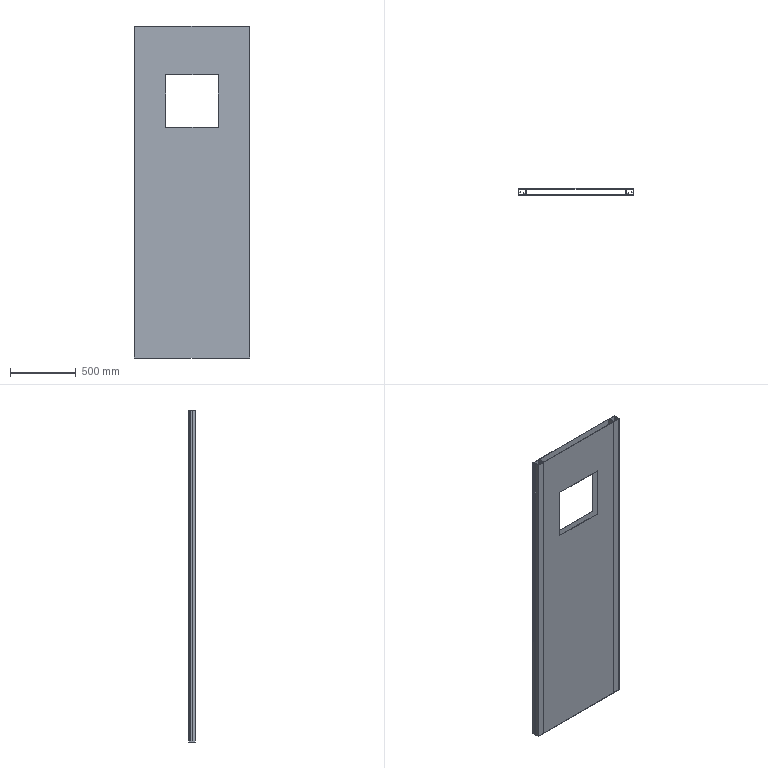Part | SolidWorks | features ICE 2, Extrusion 1 | 4 solids | 56 faces | box 880 x 51.5 x 2520 mm | volume 7151820 mm3 | plane 56